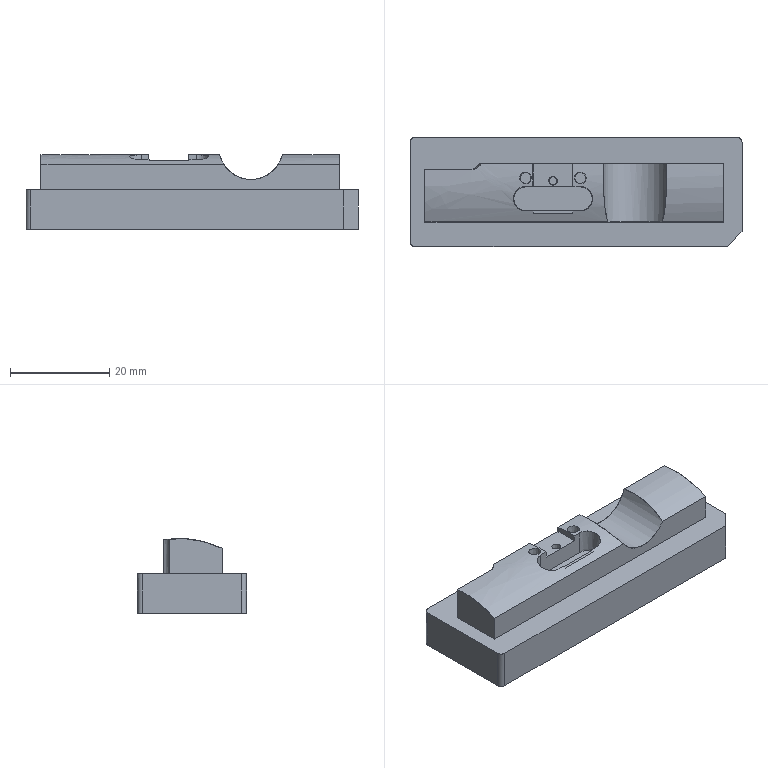NC program | PowerMill | posted with a generic post | part box 67 x 22 x 15.086 mm
Lines 46023 to 46760 of 221347:
N46120 M6
N46121 S8500 M03
N46122 G00 G90 X0.0 Y0.0
N46123 G43 Z9.7955 H3
N46124
N46125 G05 P10000 R8
N46126 X-37.453 Y-20.6584
N46127 Z-6.09
N46128 G01 Z-7.29 F360.0
N46129 X-35.1675 Y-15.9042 F600.0
N46130 X-26.2471 Y-11.444
N46131 X-30.4768
N46132 X-30.7583 Y-11.4366
N46133 X-31.0391 Y-11.4145
N46134 X-31.3184 Y-11.3778
N46135 X-31.5953 Y-11.3264
N46136 X-31.8692 Y-11.2607
N46137 X-32.1393 Y-11.1807
N46138 X-32.4048 Y-11.0867
N46139 X-32.665 Y-10.9789
N46140 X-32.9192 Y-10.8576
N46141 X-33.1668 Y-10.7232
N46142 X-33.4069 Y-10.5761
N46143 X-33.6391 Y-10.4165
N46144 X-33.8625 Y-10.2451
N46145 X-34.0767 Y-10.0621
N46146 X-34.281 Y-9.8683
N46147 X-34.4749 Y-9.6639
N46148 X-34.6578 Y-9.4498
N46149 X-34.8293 Y-9.2263
N46150 X-34.9888 Y-8.9942
N46151 X-35.136 Y-8.754
N46152 X-35.2704 Y-8.5065
N46153 X-35.3916 Y-8.2523
N46154 X-35.4994 Y-7.992
N46155 X-35.5934 Y-7.7265
N46156 X-35.6735 Y-7.4565
N46157 X-35.7392 Y-7.1826
N46158 X-35.7905 Y-6.9056
N46159 X-35.8273 Y-6.6264
N46160 X-35.8494 Y-6.3456
N46161 X-35.8568 Y-6.064
N46162 Y4.5076
N46163 X-35.8494 Y4.7891
N46164 X-35.8273 Y5.0699
N46165 X-35.7799 Y5.4063
N46166 X-35.7392 Y5.6261
N46167 X-35.6734 Y5.9
N46168 X-35.5935 Y6.1701
N46169 X-35.4994 Y6.4356
N46170 X-35.3916 Y6.6958
N46171 X-35.2704 Y6.95
N46172 X-35.136 Y7.1976
N46173 X-34.9888 Y7.4377
N46174 X-34.8293 Y7.6698
N46175 X-34.6578 Y7.8933
N46176 X-34.4749 Y8.1075
N46177 X-34.281 Y8.3118
N46178 X-34.0767 Y8.5057
N46179 X-33.8625 Y8.6886
N46180 X-33.639 Y8.8601
N46181 X-33.4069 Y9.0196
N46182 G02 X-32.9192 Y9.3012 I3.195 J-4.9712
N46183 G01 X-32.665 Y9.4224
N46184 X-32.4048 Y9.5302
N46185 X-32.1393 Y9.6242
N46186 X-31.8692 Y9.7042
N46187 X-31.5953 Y9.77
N46188 X-31.3184 Y9.8213
N46189 X-31.0391 Y9.8581
N46190 X-30.7583 Y9.8802
N46191 X-30.4768 Y9.8875
N46192 X-23.2331
N46193 G03 X-22.6665 Y10.0635 I0.0 J1.0001
N46194 G01 X-22.4407 Y10.2188
N46195 X-22.2005 Y10.3661
N46196 X-21.9528 Y10.5006
N46197 X-21.6985 Y10.622
N46198 X-21.4382 Y10.7299
N46199 X-21.1726 Y10.824
N46200 X-20.9024 Y10.9041
N46201 X-20.6284 Y10.9699
N46202 X-20.3513 Y11.0213
N46203 X-20.072 Y11.058
N46204 X-19.791 Y11.0802
N46205 X-19.5093 Y11.0876
N46206 X29.7595 Y11.0875
N46207 X30.0411 Y11.0802
N46208 X30.3219 Y11.0581
N46209 X30.6011 Y11.0213
N46210 X30.8781 Y10.97
N46211 X31.1519 Y10.9042
N46212 X31.422 Y10.8242
N46213 X31.6875 Y10.7302
N46214 X31.9477 Y10.6224
N46215 X32.202 Y10.5012
N46216 X32.4495 Y10.3668
N46217 X32.6896 Y10.2196
N46218 X32.9218 Y10.0601
N46219 X33.1452 Y9.8886
N46220 X33.3594 Y9.7057
N46221 X33.5499 Y9.5256
N46222 X33.7576 Y9.3075
N46223 X33.9405 Y9.0933
N46224 X34.112 Y8.8698
N46225 X34.2715 Y8.6377
N46226 X34.4187 Y8.3975
N46227 X34.5531 Y8.15
N46228 X34.6744 Y7.8958
N46229 X34.7822 Y7.6356
N46230 X34.8762 Y7.3701
N46231 X34.9562 Y7.1
N46232 X35.0219 Y6.8261
N46233 X35.0733 Y6.5492
N46234 X35.11 Y6.2699
N46235 X35.1321 Y5.9891
N46236 X35.1395 Y5.7075
N46237 Y-6.064
N46238 X35.1321 Y-6.3456
N46239 X35.11 Y-6.6264
N46240 X35.0732 Y-6.9056
N46241 X35.0219 Y-7.1826
N46242 X34.9562 Y-7.4565
N46243 X34.8762 Y-7.7265
N46244 X34.7822 Y-7.992
N46245 X34.6744 Y-8.2523
N46246 X34.5531 Y-8.5065
N46247 X34.4187 Y-8.754
N46248 X34.2715 Y-8.9942
N46249 X34.112 Y-9.2263
N46250 X33.9406 Y-9.4498
N46251 X33.7576 Y-9.6639
N46252 X33.5637 Y-9.8682
N46253 X33.3594 Y-10.0621
N46254 X33.1452 Y-10.2451
N46255 G02 X32.6896 Y-10.5761 I-3.7098 J4.6272
N46256 G01 X32.4495 Y-10.7232
N46257 X32.202 Y-10.8576
N46258 X31.9477 Y-10.9789
N46259 X31.6875 Y-11.0867
N46260 X31.4299 Y-11.1781
N46261 X31.1519 Y-11.2607
N46262 X30.8781 Y-11.3264
N46263 X30.6011 Y-11.3778
N46264 X30.3219 Y-11.4145
N46265 X30.0411 Y-11.4366
N46266 X29.7595 Y-11.444
N46267 X-26.2471
N46268 G00 Z9.7955
N46269 G05 P0
N46270 (---------------)
N46271 ( END TOOLPATH : 精公基准台01-基准面偏置-D10 )
N46272 (---------------)
N46273 ( START TOOLPATH : 精公基准台01-外形侧光-D10 )
N46274 (---------------)
N46275 G00 X0.0 Y0.0 Z10.795
N46276 G05 P10000 R8
N46277 X32.7713 Y-10.7276
N46278 Z-6.06
N46279 G01 Z-7.26 F360.0
N46280 G03 X31.6233 Y-10.7144 I-0.5899 J-1.3791 F600.0
N46281 G02 X29.7567 Y-11.074 I-1.8639 J4.6505
N46282 G01 X-0.3651
N46283 X-30.4886
N46284 G02 X-35.4865 Y-6.1156 I0.0119 J5.01
N46285 G01 X-35.4868 Y4.4736
N46286 G02 X-30.4869 Y9.5175 I5.0103 J0.0336
N46287 G01 X-22.8374
N46288 G03 X-22.6956 Y9.5693 I0.0 J0.22
N46289 G02 X-19.5335 Y10.7175 I3.1911 J-3.8602
N46290 G01 X0.1019
N46291 X29.7581
N46292 G02 X34.7693 Y5.7505 I0.0014 J-5.01
N46293 G01 X34.7692 Y-6.1176
N46294 G02 X31.6233 Y-10.7144 I-5.0098 J0.0536
N46295 G03 X30.8022 Y-11.5168 I0.5581 J-1.3923
N46296 G01 X32.6492 Y-10.7121
N46297 G03 X31.5017 Y-10.6759 I-0.6174 J-1.367
N46298 G02 X29.7567 Y-10.994 I-1.7422 J4.6119
N46299 G01 X-0.3651
N46300 X-30.4869
N46301 G02 X-35.4065 Y-6.1156 I0.0101 J4.93
N46302 G01 X-35.4068 Y4.4726
N46303 G02 X-30.4869 Y9.4375 I4.9303 J0.0346
N46304 G01 X-22.8374
N46305 G03 X-22.644 Y9.5082 I0.0 J0.3001
N46306 G02 X-19.5335 Y10.6375 I3.1394 J-3.7988
N46307 G01 X0.1019
N46308 X29.7567 Y10.6376
N46309 G02 X34.6893 Y5.7505 I0.0028 J-4.9301
N46310 G01 X34.6892 Y-6.1156
N46311 G02 X31.5017 Y-10.6759 I-4.9297 J0.0516
N46312 G03 X30.6647 Y-11.4617 I0.5301 J-1.4032
N46313 G00 Z10.795
N46314 G05 P0
N46315 (---------------)
N46316 ( END TOOLPATH : 精公基准台01-外形侧光-D10 )
N46317 (---------------)
N46318 ( START TOOLPATH : 精公基准台01-基准台侧光-D10 )
N46319 (---------------)
N46320 G00 X0.0 Y0.0 Z9.7955
N46321 G05 P10000 R8
N46322 X37.7574 Y-17.9979
N46323 Z-13.99
N46324 G01 Z-15.19 F360.0
N46325 G03 X34.2219 Y-14.4623 I-1.7678 J1.7678 F600.0
N46326 G01 X34.0849 Y-14.5993
N46327 X34.0841 Y-14.6001
N46328 X34.0832 Y-14.6009
N46329 X33.8825 Y-14.7901
N46330 X33.8811 Y-14.7914
N46331 X33.8797 Y-14.7927
N46332 X33.7316 Y-14.9196
N46333 X33.7303 Y-14.9206
N46334 X33.7291 Y-14.9217
N46335 X33.561 Y-15.0542
N46336 X33.5593 Y-15.0555
N46337 X33.5576 Y-15.0568
N46338 X33.2974 Y-15.2404
N46339 X33.2949 Y-15.242
N46340 X33.2924 Y-15.2436
N46341 X32.9202 Y-15.4663
N46342 X32.918 Y-15.4676
N46343 X32.9158 Y-15.4688
N46344 X32.7343 Y-15.5623
N46345 X32.733 Y-15.5629
N46346 X32.7318 Y-15.5635
N46347 X32.5971 Y-15.6269
N46348 X32.5953 Y-15.6278
N46349 X32.5935 Y-15.6285
N46350 X32.2774 Y-15.7589
N46351 X32.2746 Y-15.76
N46352 X32.2718 Y-15.7609
N46353 X31.8998 Y-15.8833
N46354 X31.8973 Y-15.8841
N46355 X31.8947 Y-15.8848
N46356 X31.6345 Y-15.9517
N46357 X31.6322 Y-15.9522
N46358 X31.6299 Y-15.9527
N46359 X31.3137 Y-16.0144
N46360 X31.3112 Y-16.0148
N46361 X31.3087 Y-16.0152
N46362 X30.9925 Y-16.056
N46363 X30.99 Y-16.0563
N46364 X30.9875 Y-16.0565
N46365 X30.6713 Y-16.0771
N46366 X30.6691 Y-16.0772
N46367 X30.6668 Y-16.0773
N46368 X30.3507 Y-16.08
N46369 X30.3503
N46370 X30.35
N46371 X-32.563 Y-16.0796
N46372 X-32.5645
N46373 X-32.5659
N46374 X-32.8821 Y-16.068
N46375 X-32.8842 Y-16.0679
N46376 X-32.8863 Y-16.0677
N46377 X-33.2025 Y-16.0392
N46378 X-33.2046 Y-16.039
N46379 X-33.2067 Y-16.0387
N46380 X-33.5228 Y-15.9933
N46381 X-33.5249 Y-15.993
N46382 X-33.5271 Y-15.9926
N46383 X-33.8432 Y-15.9297
N46384 X-33.8453 Y-15.9292
N46385 X-33.8474 Y-15.9287
N46386 X-34.1636 Y-15.8478
N46387 X-34.1657 Y-15.8473
N46388 X-34.1678 Y-15.8466
N46389 X-34.4839 Y-15.7471
N46390 X-34.486 Y-15.7464
N46391 X-34.4881 Y-15.7456
N46392 X-34.8043 Y-15.6264
N46393 X-34.8064 Y-15.6256
N46394 X-34.8085 Y-15.6247
N46395 X-35.1247 Y-15.4842
N46396 X-35.1268 Y-15.4832
N46397 X-35.1289 Y-15.4821
N46398 X-35.445 Y-15.3189
N46399 X-35.4465 Y-15.3181
N46400 X-35.4479 Y-15.3173
N46401 X-35.5759 Y-15.2445
N46402 X-35.577 Y-15.2439
N46403 X-35.5781 Y-15.2432
N46404 X-35.7663 Y-15.1279
N46405 X-35.7678 Y-15.1269
N46406 X-35.7694 Y-15.1259
N46407 X-36.0651 Y-14.925
N46408 X-36.0673 Y-14.9235
N46409 X-36.0694 Y-14.9219
N46410 X-36.406 Y-14.6593
N46411 X-36.4082 Y-14.6575
N46412 X-36.4103 Y-14.6557
N46413 X-36.7265 Y-14.3706
N46414 X-36.7278 Y-14.3694
N46415 X-36.7291 Y-14.3681
N46416 X-36.8148 Y-14.2835
N46417 X-36.8159 Y-14.2824
N46418 X-36.817 Y-14.2813
N46419 X-37.0474 Y-14.0357
N46420 X-37.0484 Y-14.0346
N46421 X-37.0495 Y-14.0334
N46422 X-37.1107 Y-13.9628
N46423 X-37.1117 Y-13.9617
N46424 X-37.1126 Y-13.9605
N46425 X-37.3666 Y-13.6444
N46426 X-37.3682 Y-13.6422
N46427 X-37.3698 Y-13.64
N46428 X-37.5904 Y-13.3239
N46429 X-37.5914 Y-13.3225
N46430 X-37.5923 Y-13.321
N46431 X-37.6889 Y-13.1689
N46432 X-37.6896 Y-13.1677
N46433 X-37.6903 Y-13.1666
N46434 X-37.7868 Y-13.0026
N46435 X-37.7877 Y-13.001
N46436 X-37.7886 Y-12.9994
N46437 X-37.9559 Y-12.6832
N46438 X-37.9569 Y-12.6811
N46439 X-37.9579 Y-12.679
N46440 X-38.102 Y-12.3629
N46441 X-38.1029 Y-12.3608
N46442 X-38.1038 Y-12.3586
N46443 X-38.2266 Y-12.0425
N46444 X-38.2274 Y-12.0404
N46445 X-38.2281 Y-12.0383
N46446 X-38.3297 Y-11.7265
N46447 X-38.3303 Y-11.7244
N46448 X-38.3309 Y-11.7223
N46449 X-38.4162 Y-11.4018
N46450 X-38.4167 Y-11.3996
N46451 X-38.4172 Y-11.3974
N46452 X-38.4825 Y-11.0813
N46453 X-38.4829 Y-11.0793
N46454 X-38.4832 Y-11.0773
N46455 X-38.5321 Y-10.7612
N46456 X-38.5324 Y-10.7589
N46457 X-38.5327 Y-10.7567
N46458 X-38.5634 Y-10.4406
N46459 X-38.5636 Y-10.4386
N46460 X-38.5637 Y-10.4366
N46461 X-38.5786 Y-10.1204
N46462 Y-10.1187
N46463 X-38.5787 Y-10.117
N46464 X-38.58 Y-9.8009
N46465 Y-9.8007
N46466 Y-9.8005
N46467 Y9.8005
N46468 Y9.8007
N46469 Y9.8009
N46470 X-38.5787 Y10.117
N46471 X-38.5786 Y10.1186
N46472 Y10.1203
N46473 X-38.5643 Y10.4364
N46474 X-38.5641 Y10.4386
N46475 X-38.564 Y10.4407
N46476 X-38.5327 Y10.7568
N46477 X-38.5324 Y10.7589
N46478 X-38.5321 Y10.761
N46479 X-38.4838 Y11.0772
N46480 X-38.4834 Y11.0793
N46481 X-38.483 Y11.0814
N46482 X-38.4172 Y11.3976
N46483 X-38.4167 Y11.3997
N46484 X-38.4162 Y11.4018
N46485 X-38.3322 Y11.7179
N46486 X-38.3316 Y11.7201
N46487 X-38.3309 Y11.7222
N46488 X-38.2278 Y12.0383
N46489 X-38.2271 Y12.0404
N46490 X-38.2263 Y12.0424
N46491 X-38.1038 Y12.3586
N46492 X-38.1029 Y12.3608
N46493 X-38.102 Y12.3629
N46494 X-37.9576 Y12.6791
N46495 X-37.9566 Y12.6811
N46496 X-37.9555 Y12.6832
N46497 X-37.7886 Y12.9993
N46498 X-37.7878 Y13.0009
N46499 X-37.7868 Y13.0026
N46500 X-37.6903 Y13.1666
N46501 X-37.6896 Y13.1677
N46502 X-37.689 Y13.1687
N46503 X-37.5929 Y13.3208
N46504 X-37.5919 Y13.3224
N46505 X-37.5908 Y13.324
N46506 X-37.3708 Y13.6388
N46507 X-37.3692 Y13.6409
N46508 X-37.3676 Y13.643
N46509 X-37.113 Y13.9605
N46510 X-37.112 Y13.9617
N46511 X-37.1109 Y13.963
N46512 X-37.0493 Y14.0336
N46513 X-37.0484 Y14.0347
N46514 X-37.0474 Y14.0357
N46515 X-36.817 Y14.2813
N46516 X-36.8159 Y14.2824
N46517 X-36.8148 Y14.2835
N46518 X-36.7291 Y14.3681
N46519 X-36.728 Y14.3691
N46520 X-36.7268 Y14.3702
N46521 X-36.4732 Y14.6018
N46522 X-36.4712 Y14.6036
N46523 X-36.4691 Y14.6053
N46524 X-36.0904 Y14.9066
N46525 X-36.0881 Y14.9084
N46526 X-36.0857 Y14.9101
N46527 X-35.7696 Y15.1258
N46528 X-35.7679 Y15.1269
N46529 X-35.7663 Y15.1279
N46530 X-35.5781 Y15.2432
N46531 X-35.577 Y15.2439
N46532 X-35.5759 Y15.2445
N46533 X-35.4479 Y15.3173
N46534 X-35.4465 Y15.3181
N46535 X-35.445 Y15.3189
N46536 X-35.1289 Y15.4822
N46537 X-35.1268 Y15.4833
N46538 X-35.1246 Y15.4843
N46539 X-34.8085 Y15.6247
N46540 X-34.8064 Y15.6256
N46541 X-34.8043 Y15.6264
N46542 X-34.4881 Y15.7457
N46543 X-34.486 Y15.7465
N46544 X-34.4839 Y15.7472
N46545 X-34.1677 Y15.8467
N46546 X-34.1657 Y15.8473
N46547 X-34.1636 Y15.8479
N46548 X-33.8474 Y15.9288
N46549 X-33.8452 Y15.9293
N46550 X-33.843 Y15.9298
N46551 X-33.5269 Y15.9919
N46552 X-33.5249 Y15.9922
N46553 X-33.523 Y15.9925
N46554 X-33.2068 Y16.0387
N46555 X-33.2045 Y16.039
N46556 X-33.2022 Y16.0392
N46557 X-32.8861 Y16.0668
N46558 X-32.8842 Y16.0669
N46559 X-32.8823 Y16.067
N46560 X-32.5662 Y16.0796
N46561 X-32.5646
N46562 X-32.563
N46563 X0.0
N46564 X32.563
N46565 X32.5645
N46566 X32.5659
N46567 X32.8821 Y16.068
N46568 X32.8842 Y16.0679
N46569 X32.8863 Y16.0677
N46570 X33.2025 Y16.0392
N46571 X33.2046 Y16.039
N46572 X33.2067 Y16.0387
N46573 X33.5228 Y15.9933
N46574 X33.5249 Y15.993
N46575 X33.5271 Y15.9926
N46576 X33.8432 Y15.9297
N46577 X33.8453 Y15.9292
N46578 X33.8474 Y15.9287
N46579 X34.1636 Y15.8478
N46580 X34.1657 Y15.8473
N46581 X34.1678 Y15.8466
N46582 X34.4839 Y15.7471
N46583 X34.486 Y15.7464
N46584 X34.4881 Y15.7456
N46585 X34.8043 Y15.6264
N46586 X34.8064 Y15.6256
N46587 X34.8085 Y15.6247
N46588 X35.1247 Y15.4842
N46589 X35.1268 Y15.4832
N46590 X35.1289 Y15.4821
N46591 X35.445 Y15.3189
N46592 X35.4465 Y15.3181
N46593 X35.4479 Y15.3173
N46594 X35.5759 Y15.2445
N46595 X35.577 Y15.2439
N46596 X35.5781 Y15.2432
N46597 X35.7663 Y15.1279
N46598 X35.7678 Y15.1269
N46599 X35.7694 Y15.1259
N46600 X36.0651 Y14.925
N46601 X36.0673 Y14.9235
N46602 X36.0694 Y14.9219
N46603 X36.406 Y14.6593
N46604 X36.4082 Y14.6575
N46605 X36.4103 Y14.6557
N46606 X36.7265 Y14.3706
N46607 X36.7278 Y14.3694
N46608 X36.7291 Y14.3681
N46609 X36.8148 Y14.2835
N46610 X36.8159 Y14.2824
N46611 X36.817 Y14.2813
N46612 X37.0474 Y14.0357
N46613 X37.0484 Y14.0346
N46614 X37.0495 Y14.0334
N46615 X37.1107 Y13.9628
N46616 X37.1117 Y13.9617
N46617 X37.1126 Y13.9605
N46618 X37.3666 Y13.6444
N46619 X37.3682 Y13.6422
N46620 X37.3698 Y13.64
N46621 X37.5904 Y13.3239
N46622 X37.5914 Y13.3225
N46623 X37.5923 Y13.321
N46624 X37.6889 Y13.1689
N46625 X37.6896 Y13.1677
N46626 X37.6903 Y13.1666
N46627 X37.7868 Y13.0026
N46628 X37.7877 Y13.001
N46629 X37.7886 Y12.9994
N46630 X37.9559 Y12.6832
N46631 X37.9569 Y12.6811
N46632 X37.9579 Y12.679
N46633 X38.102 Y12.3629
N46634 X38.1029 Y12.3608
N46635 X38.1038 Y12.3586
N46636 X38.2266 Y12.0425
N46637 X38.2274 Y12.0404
N46638 X38.2281 Y12.0383
N46639 X38.3297 Y11.7265
N46640 X38.3303 Y11.7244
N46641 X38.3309 Y11.7223
N46642 X38.4162 Y11.4018
N46643 X38.4167 Y11.3996
N46644 X38.4172 Y11.3974
N46645 X38.4825 Y11.0813
N46646 X38.4829 Y11.0793
N46647 X38.4832 Y11.0773
N46648 X38.5321 Y10.7612
N46649 X38.5324 Y10.7589
N46650 X38.5327 Y10.7567
N46651 X38.5634 Y10.4406
N46652 X38.5636 Y10.4386
N46653 X38.5637 Y10.4366
N46654 X38.5786 Y10.1204
N46655 Y10.1187
N46656 X38.5787 Y10.117
N46657 X38.58 Y9.8009
N46658 Y9.8007
N46659 Y9.8005
N46660 Y-7.9036
N46661 Y-7.9043
N46662 Y-7.9049
N46663 X38.5752 Y-8.221
N46664 X38.5751 Y-8.2234
N46665 X38.575 Y-8.2258
N46666 X38.551 Y-8.542
N46667 X38.5507 Y-8.5445
N46668 X38.5504 Y-8.547
N46669 X38.5061 Y-8.8632
N46670 X38.5057 Y-8.8657
N46671 X38.5052 Y-8.8682
N46672 X38.44 Y-9.1844
N46673 X38.4394 Y-9.1869
N46674 X38.4388 Y-9.1895
N46675 X38.3517 Y-9.5056
N46676 X38.351 Y-9.5081
N46677 X38.3502 Y-9.5107
N46678 X38.2401 Y-9.8268
N46679 X38.2392 Y-9.8294
N46680 X38.2382 Y-9.8319
N46681 X38.1035 Y-10.148
N46682 X38.1026 Y-10.15
N46683 X38.1016 Y-10.152
N46684 X38.0092 Y-10.3395
N46685 X38.0086 Y-10.3407
N46686 X38.0079 Y-10.342
N46687 X37.9387 Y-10.4707
N46688 X37.9377 Y-10.4725
N46689 X37.9366 Y-10.4743
N46690 X37.7449 Y-10.7904
N46691 X37.7439 Y-10.792
N46692 X37.7429 Y-10.7936
N46693 X37.6877 Y-10.8757
N46694 X37.6868 Y-10.8769
N46695 X37.6859 Y-10.8782
N46696 X37.5149 Y-11.1123
N46697 X37.5137 Y-11.114
N46698 X37.5124 Y-11.1156
N46699 X37.3672 Y-11.294
N46700 X37.3662 Y-11.2953
N46701 X37.3651 Y-11.2966
N46702 X37.2433 Y-11.4342
N46703 X37.2421 Y-11.4356
N46704 X37.2409 Y-11.4369
N46705 X37.0465 Y-11.6377
N46706 X37.0461 Y-11.6381
N46707 X37.0456 Y-11.6386
N46708 X34.2219 Y-14.4623
N46709 G03 X37.7574 Y-17.9979 I1.7677 J-1.7678
N46710 G01 X37.7116 Y-17.9305
N46711 G03 X34.1761 Y-14.395 I-1.7677 J1.7678
N46712 G01 X34.0284 Y-14.5427
N46713 X33.8276 Y-14.7319
N46714 X33.6795 Y-14.8588
N46715 X33.5114 Y-14.9914
N46716 X33.2513 Y-15.175
N46717 X32.8792 Y-15.3977
N46718 X32.6977 Y-15.4911
N46719 X32.563 Y-15.5546
N46720 X32.2469 Y-15.6849
N46721 X31.8748 Y-15.8073
N46722 X31.6146 Y-15.8742
N46723 X31.2984 Y-15.9359
N46724 X30.9823 Y-15.9767
N46725 X30.6661 Y-15.9973
N46726 X30.35 Y-16.0
N46727 X-32.563 Y-15.9996
N46728 X-32.8792 Y-15.988
N46729 X-33.1953 Y-15.9595
N46730 X-33.5114 Y-15.9141
N46731 X-33.8276 Y-15.8512
N46732 X-34.1437 Y-15.7703
N46733 X-34.4599 Y-15.6708
N46734 X-34.776 Y-15.5516
N46735 X-35.0922 Y-15.4111
N46736 X-35.4083 Y-15.2478
N46737 X-35.5363 Y-15.175
N46738 X-35.7245 Y-15.0597
N46739 X-36.0202 Y-14.8588
N46740 X-36.3568 Y-14.5963
N46741 X-36.6729 Y-14.3112
N46742 X-36.7587 Y-14.2266
N46743 X-36.989 Y-13.981
N46744 X-37.0503 Y-13.9104
N46745 X-37.3042 Y-13.5943
N46746 X-37.5248 Y-13.2781
N46747 X-37.6213 Y-13.126
N46748 X-37.7179 Y-12.962
N46749 X-37.8851 Y-12.6458
N46750 X-38.0292 Y-12.3297
N46751 X-38.152 Y-12.0135
N46752 X-38.2536 Y-11.7017
N46753 X-38.3388 Y-11.3812
N46754 X-38.4041 Y-11.0651
N46755 X-38.4531 Y-10.749
N46756 X-38.4838 Y-10.4328
N46757 X-38.4987 Y-10.1167
N46758 X-38.5 Y-9.8005
N46759 Y9.8005
N46760 X-38.4987 Y10.1167
N46761 X-38.4844 Y10.4328
N46762 X-38.4531 Y10.749
N46763 X-38.4047 Y11.0651
N46764 X-38.3388 Y11.3812
N46765 X-38.2549 Y11.6974
N46766 X-38.1518 Y12.0135
N46767 X-38.0292 Y12.3297
N46768 X-37.8848 Y12.6458
N46769 X-37.7179 Y12.962
N46770 X-37.6213 Y13.126
N46771 X-37.5252 Y13.2781
N46772 X-37.3052 Y13.5929
N46773 X-37.0506 Y13.9104
N46774 X-36.989 Y13.981
N46775 X-36.7587 Y14.2266
N46776 X-36.6729 Y14.3111
N46777 X-36.4193 Y14.5427
N46778 X-36.0406 Y14.844
N46779 X-35.7245 Y15.0597
N46780 X-35.5363 Y15.175
N46781 X-35.4083 Y15.2478
N46782 X-35.0922 Y15.4112
N46783 X-34.776 Y15.5516
N46784 X-34.4599 Y15.6709
N46785 X-34.1437 Y15.7704
N46786 X-33.8276 Y15.8513
N46787 X-33.5114 Y15.9134
N46788 X-33.1953 Y15.9595
N46789 X-32.8792 Y15.9871
N46790 X-32.563 Y15.9996
N46791 X0.0
N46792 X32.563
N46793 X32.8792 Y15.988
N46794 X33.1953 Y15.9595
N46795 X33.5114 Y15.9141
N46796 X33.8276 Y15.8512
N46797 X34.1437 Y15.7703
N46798 X34.4599 Y15.6708
N46799 X34.776 Y15.5516
N46800 X35.0922 Y15.4111
N46801 X35.4083 Y15.2478
N46802 X35.5363 Y15.175
N46803 X35.7245 Y15.0597
N46804 X36.0202 Y14.8588
N46805 X36.3568 Y14.5963
N46806 X36.6729 Y14.3112
N46807 X36.7587 Y14.2266
N46808 X36.989 Y13.981
N46809 X37.0503 Y13.9104
N46810 X37.3042 Y13.5943
N46811 X37.5248 Y13.2781
N46812 X37.6213 Y13.126
N46813 X37.7179 Y12.962
N46814 X37.8851 Y12.6458
N46815 X38.0292 Y12.3297
N46816 X38.152 Y12.0135
N46817 X38.2536 Y11.7017
N46818 X38.3388 Y11.3812
N46819 X38.4041 Y11.0651
N46820 X38.4531 Y10.749
N46821 X38.4838 Y10.4328
N46822 X38.4987 Y10.1167
N46823 X38.5 Y9.8005
N46824 Y-7.9036
N46825 X38.4952 Y-8.2198
N46826 X38.4712 Y-8.5359
N46827 X38.4269 Y-8.8521
N46828 X38.3616 Y-9.1682
N46829 X38.2746 Y-9.4844
N46830 X38.1646 Y-9.8005
N46831 X38.0299 Y-10.1167
N46832 X37.9375 Y-10.3041
N46833 X37.8682 Y-10.4328
N46834 X37.6765 Y-10.749
N46835 X37.6213 Y-10.831
N46836 X37.4503 Y-11.0651
N46837 X37.3052 Y-11.2436
N46838 X37.1834 Y-11.3812
N46839 X36.989 Y-11.582
N46840 X34.1761 Y-14.395
N46841 G03 X37.7116 Y-17.9305 I1.7678 J-1.7677
N46842 G00 Z9.7955
N46843 G05 P0
N46844 (---------------)
N46845 ( END TOOLPATH : 精公基准台01-基准台侧光-D10 )
N46846 (---------------)
N46847
N46848 M05
N46849 G53 Z0.0
N46850 (---------------)
N46851 ( START TOOLPATH : 精公精光01-平行-R1.5 )
N46852 (---------------)
N46853 ( TOOL NO.    :22 )
N46854 ( TOOL TYPE   : BALLNOSED)
N46855 ( TOOL ID     : R1.5_1_1)
N46856 ( TOOL DIA    : 3.0 LENGTH 60.28)
N46857 T22